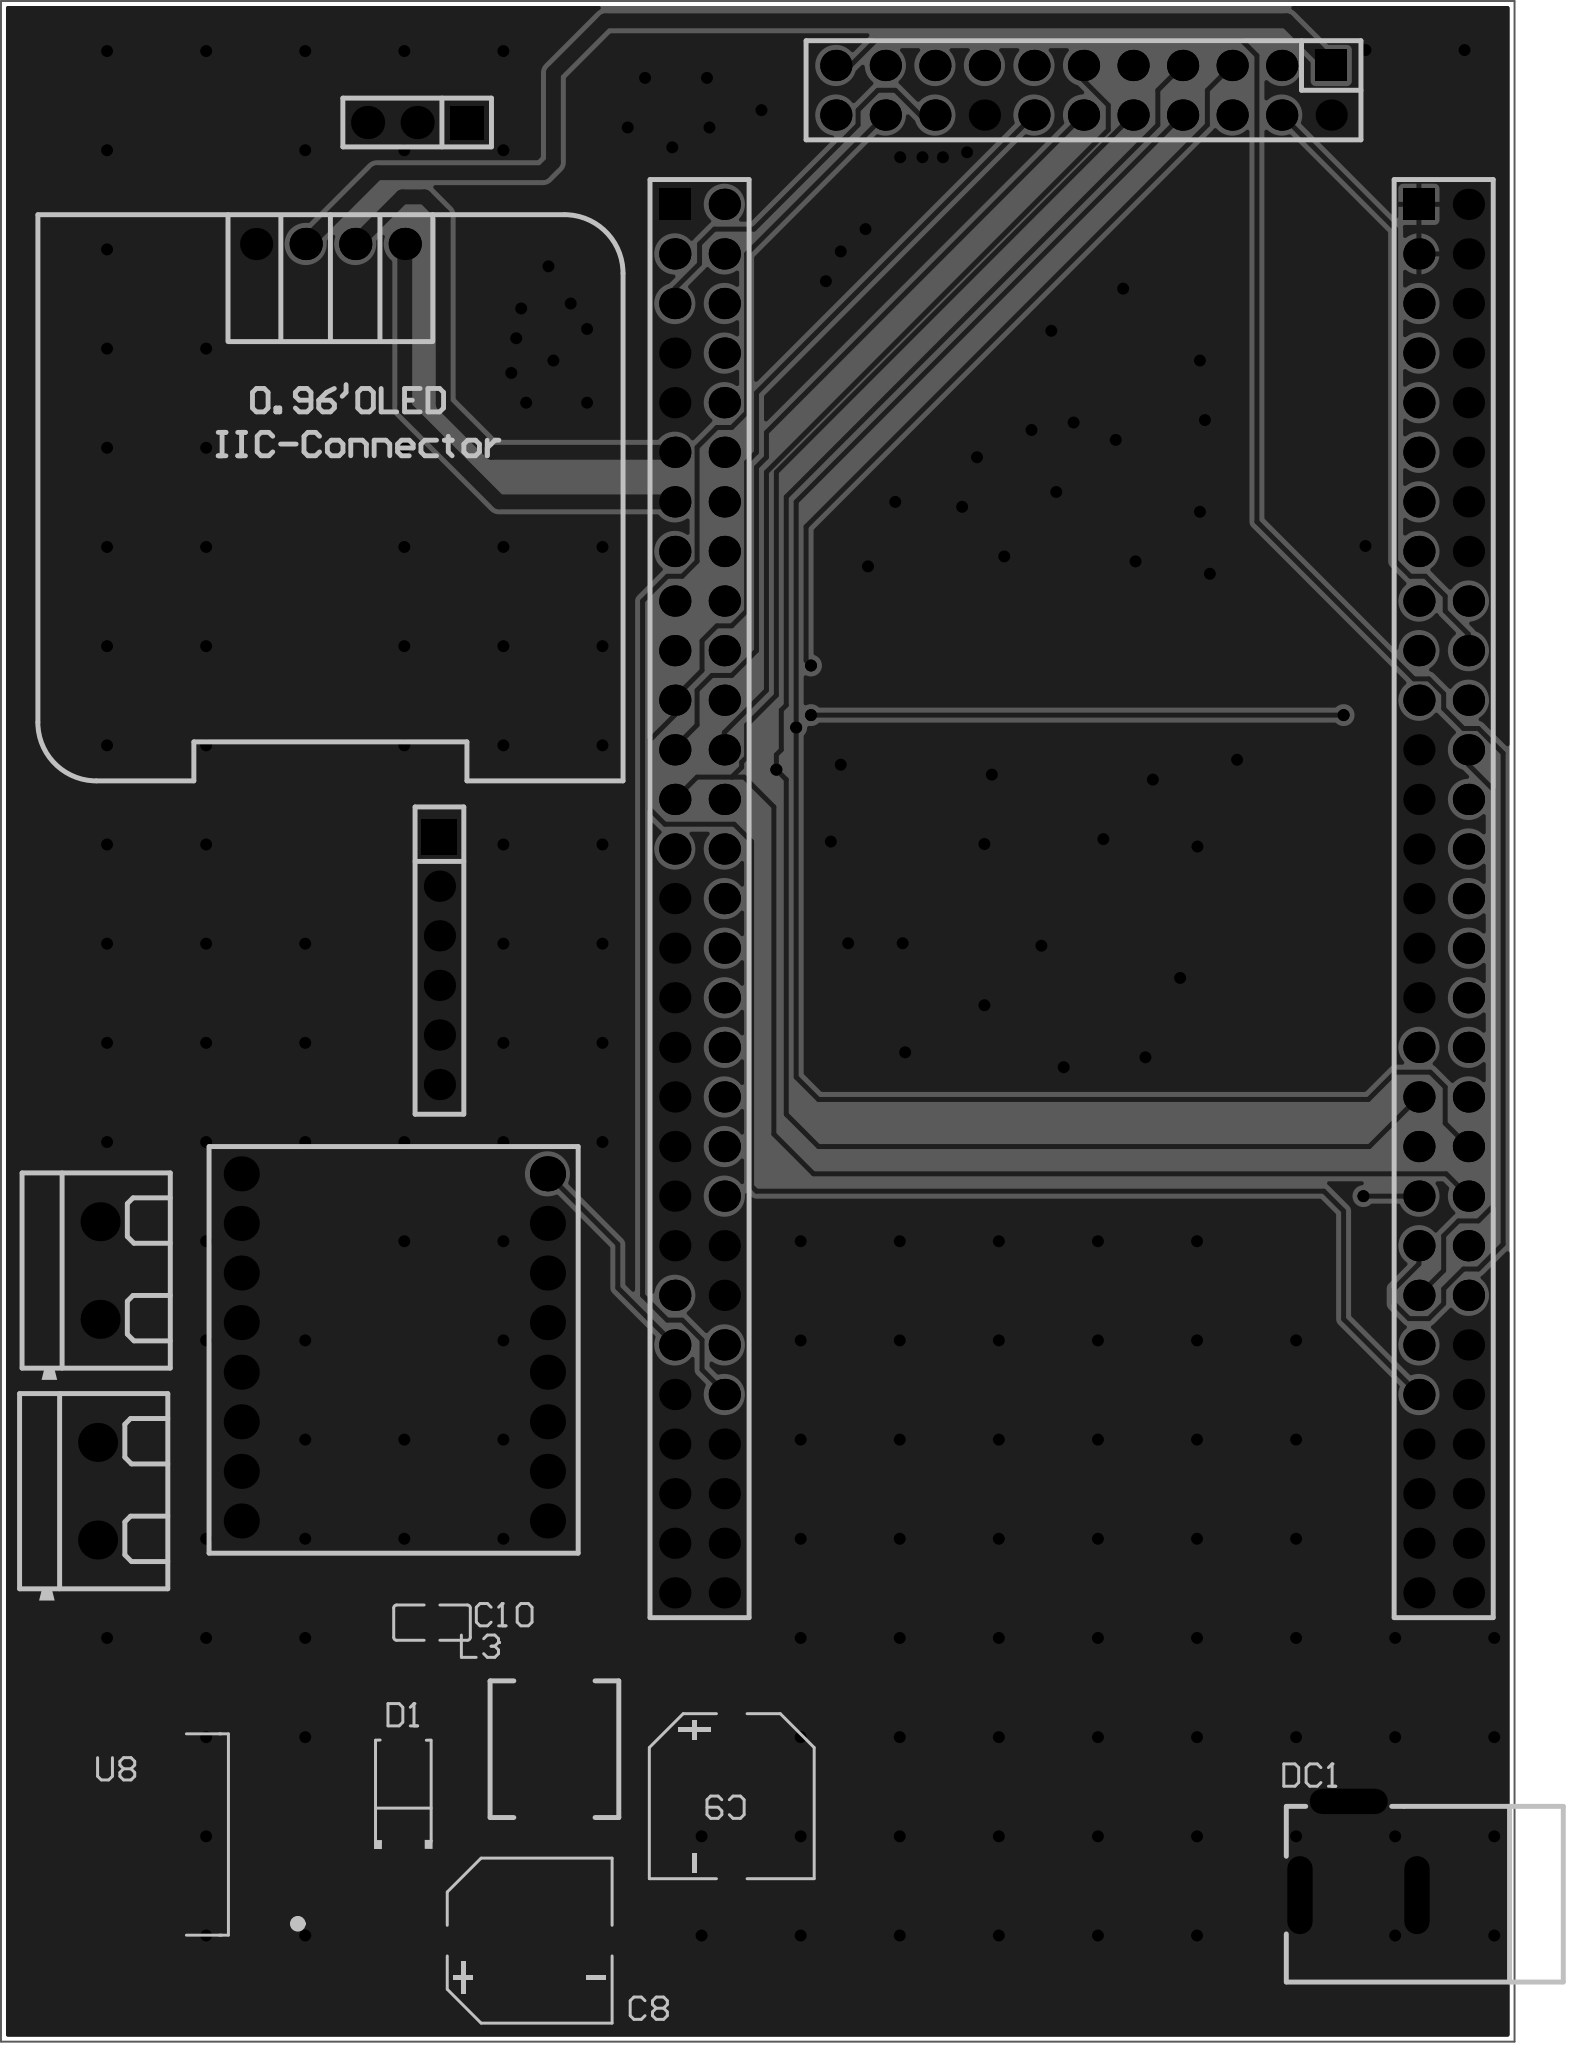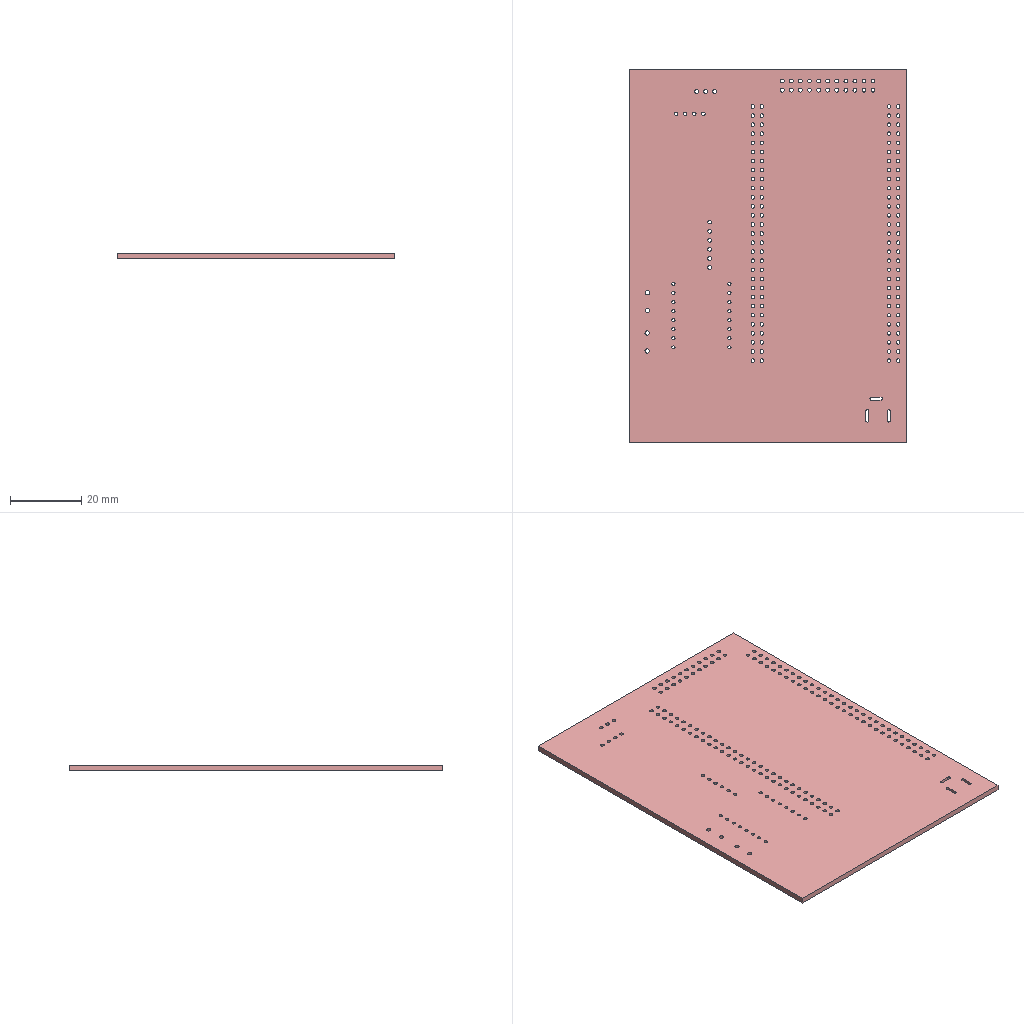Circuit board layout | Altium Designer | box 77.6 x 104.5 x 1.6 mm
Layer stack:
# Altium Designer layer stack of  (unit mm; dielectric type: 0 none, 1 core, 2 prepreg, 3 surface material)
index,name,kind,layer,copper_thickness_mm,dielectric_type,dielectric_thickness_mm,dielectric_material,dielectric_constant
0,Top Paste Mask Layer,other,,,,,,
1,Top Silkscreen Layer,other,,,,,,
2,Top Solder Mask Layer,dielectric,,,3,0.01,,3.3
3,Top Layer,copper,Top Layer,0.035,,,,
4,Dielectric1,dielectric,,,3,1.51,FR4,4.5
5,Bottom Layer,copper,Bottom Layer,0.035,,,,
6,Bottom Solder Mask Layer,dielectric,,,3,0.01,,3.3
7,Bottom Silkscreen Layer,other,,,,,,
8,Bottom Paste Mask Layer,other,,,,,,
# drill layer pairs: low layer,high layer
drill_pair,Top Layer,Bottom Layer
Part placement:
Designator,Comment,Layer,Footprint,Center-X(mm),Center-Y(mm),Rotation
H1,,TopLayer,HDR-TH_3P-P2.54-V-M,101.854,179.705,180
H4,,TopLayer,HDR-TH_6P-P2.54-V-F,102.997,136.779,270
H12,DS1023-2*11SF11,TopLayer,HDR-TH_22P-P2.54-V-F-R2-C11-S2.54,136.017,181.356,180
OLED1,,TopLayer,0.96OLED_4P,97.409,173.482,0
P1,KF301-2P接线端子,TopLayer,CONN-TH_XY301V-A-5.0-2P,85.598,120.904,270
P2,KF301-2P接线端子,TopLayer,CONN-TH_XY301V-A-5.0-2P,85.471,109.601,270
U1,KH-2.54FH-2X29P-H8.5,TopLayer,HDR-TH_58P-P2.54-V-F-R2-C29-S2.54,116.332,139.954,270
U2,KH-2.54FH-2X29P-H8.5,TopLayer,HDR-TH_58P-P2.54-V-F-R2-C29-S2.54,154.482,139.954,270
U4,,TopLayer,tb6612,100.686,116.967,0
U8,LM2596S-5.0,TopLayer,TO-263-5_L10.2-W8.9-P1.70-BR,90.677,92.018,0
C10,,TopLayer,C0805,102.616,102.87,180
D1,,TopLayer,SMA_L4.3-W2.6-LS5.2-RD,101.146,94.253,90
C9,,TopLayer,CAP-SMD_BD8.0-L8.3-W8.3-RD,117.983,93.98,90
C8,,TopLayer,CAP-SMD_BD8.0-L8.3-W8.3-RD,107.623,86.582,180
L3,,TopLayer,IND-SMD_L7.0-W6.6,108.893,96.387,90
DC1,,TopLayer,DC-2.0,150.114,91.313,0
Pad and via stacks:
# Altium Designer via and pad stacks of  (unit mm). Each distinct definition once, with the count of objects using it.
# via: kind,start_layer,end_layer,hole_mm,diameter_mm,mode(0 simple;1 top-mid-bottom;2 full stack),diameter_per_layer,count,example_net
# pad: kind,layer,hole_mm,hole_type(0 round;1 square;2 slot),plating,top_size,top_shape(1 round;2 rect;3 octagon;9 rounded rect),mid_size,bottom_size,mode,footprint,size_per_layer,count,example
pad,Multi-Layer,1.1,0,plated,1.7x1.7,2,1.7x1.7,1.7x1.7,0,HDR-TH_3P-P2.54-V-M,,1,H1.1
pad,Multi-Layer,1.1,0,plated,1.7x1.7,1,1.7x1.7,1.7x1.7,0,HDR-TH_3P-P2.54-V-M,,2,H1.2
pad,Multi-Layer,1.02,0,plated,1.6x1.6,1,1.6x1.6,1.6x1.6,0,HDR-TH_6P-P2.54-V-F,,5,H4.6
pad,Multi-Layer,1.02,0,plated,1.8x1.8,2,1.8x1.8,1.8x1.8,0,HDR-TH_6P-P2.54-V-F,,1,H4.1
pad,Multi-Layer,1.05,0,plated,1.6x1.6,2,1.6x1.6,1.6x1.6,0,HDR-TH_22P-P2.54-V-F-R2-C11-S2.54,,1,H12.1
pad,Multi-Layer,1.05,0,plated,1.6x1.6,1,1.6x1.6,1.6x1.6,0,HDR-TH_22P-P2.54-V-F-R2-C11-S2.54,,21,H12.2
pad,Multi-Layer,1,0,plated,1.65x1.65,1,1.65x1.65,1.65x1.65,0,0.96OLED_4P,,4,OLED1.4
pad,Multi-Layer,1.2,0,plated,2x2,1,2x2,2x2,0,CONN-TH_XY301V-A-5.0-2P,,4,P1.1
pad,Multi-Layer,1,0,plated,1.6x1.6,1,1.6x1.6,1.6x1.6,0,HDR-TH_58P-P2.54-V-F-R2-C29-S2.54,,114,U1.58
pad,Multi-Layer,1,0,plated,1.6x1.6,2,1.6x1.6,1.6x1.6,0,HDR-TH_58P-P2.54-V-F-R2-C29-S2.54,,2,U1.1
pad,Multi-Layer,0.9,0,plated,1.8x1.8,1,1.8x1.8,1.8x1.8,0,tb6612,,16,U4.1
pad,Multi-Layer,0.8001,2,plated,4x1.3,1,4x1.3,4x1.3,0,DC-2.0,,3,DC1.2
pad,Top Layer,0,0,plated,3.083x1.02,2,3.083x1.02,3.083x1.02,0,TO-263-5_L10.2-W8.9-P1.70-BR,,5,U8.1
pad,Top Layer,0,0,plated,8.5x11,2,8.5x11,8.5x11,0,TO-263-5_L10.2-W8.9-P1.70-BR,,1,U8.6
pad,Top Layer,0,0,plated,1.41x1.35,2,1.41x1.35,1.41x1.35,0,C0805,,2,C10.2
pad,Top Layer,0,0,plated,2x2,2,2x2,2x2,0,SMA_L4.3-W2.6-LS5.2-RD,,2,D1.2
pad,Top Layer,0,0,plated,3.61x1.26,2,3.61x1.26,3.61x1.26,0,CAP-SMD_BD8.0-L8.3-W8.3-RD,,4,C9.1
pad,Top Layer,0,0,plated,2.799x3.701,2,2.799x3.701,2.799x3.701,0,IND-SMD_L7.0-W6.6,,2,L3.1
via,Top Layer,Bottom Layer,0.3048,0.61,0,,191,B8
Copper pours:
name,layer,net,type(0 solid;1 hatched;2 none)
Bottom Layer-GND,Bottom Layer,GND,0
Top Layer-GND,Top Layer,GND,0